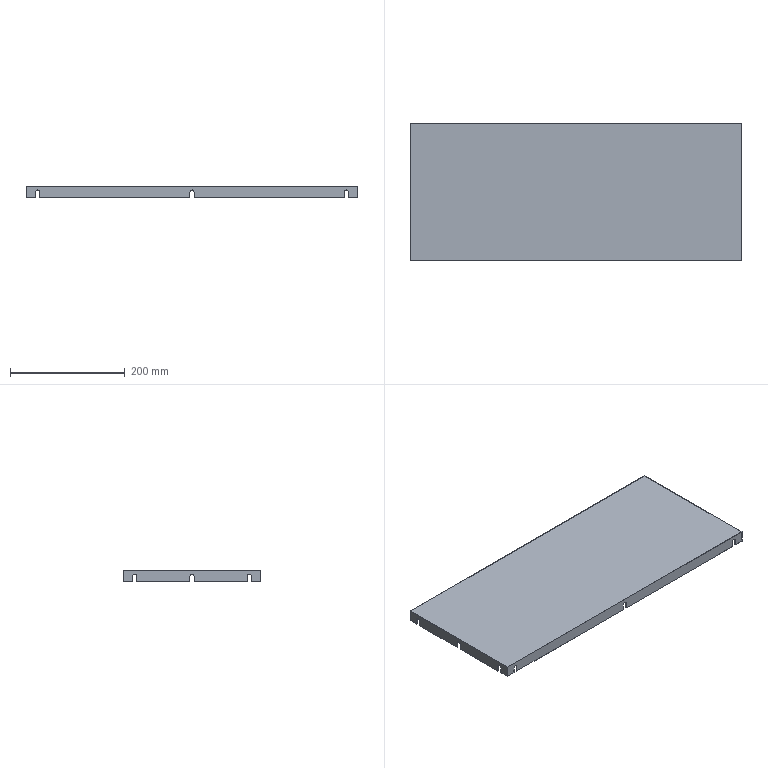Part | STEP file | 1 solid | 64 faces | box 578 x 240 x 20 mm | volume 168657 mm3 | plane 46 | cylinder 18 | commonest cylinder face diameters 7 x18